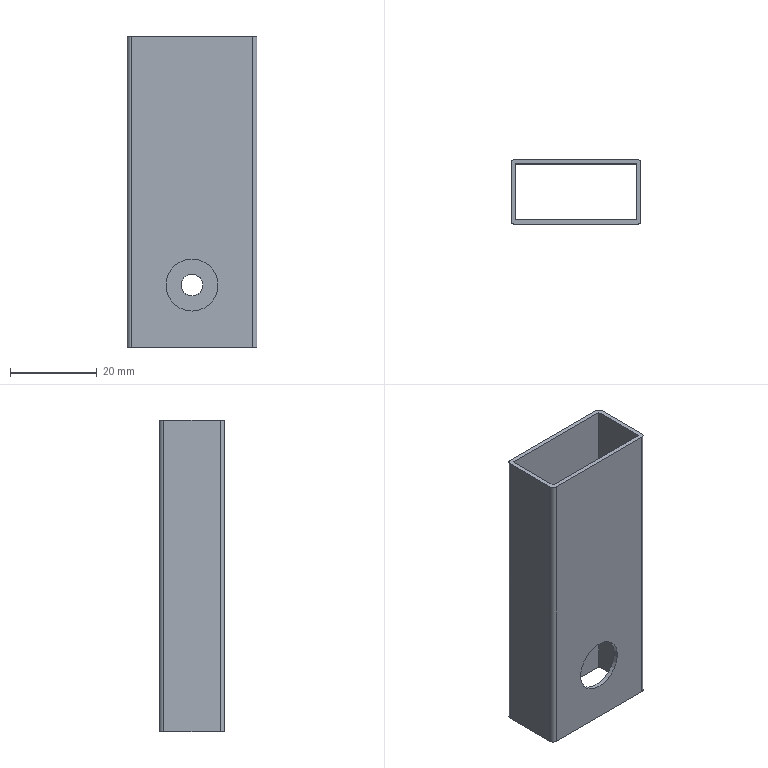Part | STEP file | Q7C1201 | 1 solid | 16 faces | box 30 x 15 x 72 mm | volume 5997 mm3 | plane 10 | cylinder 6 | commonest cylinder face diameters 2 x4 5 x1 12 x1
STEP:
#1=CARTESIAN_POINT('',(0.,0.,0.));
#2=DIRECTION('',(0.,0.,1.));
#3=DIRECTION('',(1.,0.,0.));
#4=AXIS2_PLACEMENT_3D('',#1,#2,#3);
#5=CARTESIAN_POINT('',(15.,6.5,36.));
#6=VERTEX_POINT('',#5);
#7=CARTESIAN_POINT('',(14.,7.5,36.));
#8=VERTEX_POINT('',#7);
#9=CARTESIAN_POINT('',(14.,6.5,36.));
#10=DIRECTION('',(0.,0.,1.));
#11=DIRECTION('',(-1.,0.,0.));
#12=AXIS2_PLACEMENT_3D('',#9,#10,#11);
#13=CIRCLE('',#12,1.);
#14=CARTESIAN_POINT('',(14.,6.5,36.));
#15=DIRECTION('',(0.,0.,-1.));
#16=DIRECTION('',(-1.,0.,0.));
#17=AXIS2_PLACEMENT_3D('',#14,#15,#16);
#18=PLANE('',#17);
#19=CARTESIAN_POINT('',(1.,0.));
#20=CARTESIAN_POINT('',(1.,-1.732));
#21=CARTESIAN_POINT('',(-0.5,-0.866));
#22=CARTESIAN_POINT('',(-2.,0.));
#23=CARTESIAN_POINT('',(-0.5,0.866));
#24=CARTESIAN_POINT('',(1.,1.732));
#25=CARTESIAN_POINT('',(1.,0.));
#26=(BOUNDED_CURVE()B_SPLINE_CURVE(2,(#19,#20,#21,#22,#23,#24,#25),.UNSPECIFIED.,.T.,.F.)B_SPLINE_CURVE_WITH_KNOTS((1,2,2,2,2,1),(-2.094,0.,2.094,4.189,6.283,8.378),.UNSPECIFIED.)CURVE()GEOMETRIC_REPRESENTATION_ITEM()RATIONAL_B_SPLINE_CURVE((1.,0.5,1.,0.5,1.,0.5,1.))REPRESENTATION_ITEM(''));
#27=(GEOMETRIC_REPRESENTATION_CONTEXT(2)PARAMETRIC_REPRESENTATION_CONTEXT()REPRESENTATION_CONTEXT('',''));
#28=DEFINITIONAL_REPRESENTATION('',(#26),#27);
#29=PCURVE('',#18,#28);
#30=CARTESIAN_POINT('',(14.,6.5,36.));
#31=DIRECTION('',(0.,0.,-1.));
#32=DIRECTION('',(-1.,0.,0.));
#33=AXIS2_PLACEMENT_3D('',#30,#31,#32);
#34=CYLINDRICAL_SURFACE('',#33,1.);
#35=CARTESIAN_POINT('',(6.283,0.));
#36=DIRECTION('',(-1.,0.));
#37=VECTOR('',#36,1.);
#38=LINE('',#35,#37);
#39=(GEOMETRIC_REPRESENTATION_CONTEXT(2)PARAMETRIC_REPRESENTATION_CONTEXT()REPRESENTATION_CONTEXT('',''));
#40=DEFINITIONAL_REPRESENTATION('',(#38),#39);
#41=PCURVE('',#34,#40);
#42=SURFACE_CURVE('',#13,(#29,#41),.PCURVE_S1.);
#43=EDGE_CURVE('',#6,#8,#42,.T.);
#44=ORIENTED_EDGE('',*,*,#43,.T.);
#45=CARTESIAN_POINT('',(-14.,7.5,36.));
#46=VERTEX_POINT('',#45);
#47=CARTESIAN_POINT('',(-14.,7.5,36.));
#48=DIRECTION('',(-1.,0.,0.));
#49=VECTOR('',#48,1.);
#50=LINE('',#47,#49);
#51=CARTESIAN_POINT('',(28.,1.));
#52=DIRECTION('',(1.,0.));
#53=VECTOR('',#52,1.);
#54=LINE('',#51,#53);
#55=(GEOMETRIC_REPRESENTATION_CONTEXT(2)PARAMETRIC_REPRESENTATION_CONTEXT()REPRESENTATION_CONTEXT('',''));
#56=DEFINITIONAL_REPRESENTATION('',(#54),#55);
#57=PCURVE('',#18,#56);
#58=CARTESIAN_POINT('',(-14.,7.5,36.));
#59=DIRECTION('',(0.,-1.,0.));
#60=DIRECTION('',(0.,0.,-1.));
#61=AXIS2_PLACEMENT_3D('',#58,#59,#60);
#62=PLANE('',#61);
#63=CARTESIAN_POINT('',(0.,0.));
#64=DIRECTION('',(0.,-1.));
#65=VECTOR('',#64,1.);
#66=LINE('',#63,#65);
#67=(GEOMETRIC_REPRESENTATION_CONTEXT(2)PARAMETRIC_REPRESENTATION_CONTEXT()REPRESENTATION_CONTEXT('',''));
#68=DEFINITIONAL_REPRESENTATION('',(#66),#67);
#69=PCURVE('',#62,#68);
#70=SURFACE_CURVE('',#50,(#57,#69),.PCURVE_S1.);
#71=EDGE_CURVE('',#8,#46,#70,.T.);
#72=ORIENTED_EDGE('',*,*,#71,.T.);
#73=CARTESIAN_POINT('',(-15.,6.5,36.));
#74=VERTEX_POINT('',#73);
#75=CARTESIAN_POINT('',(-14.,6.5,36.));
#76=DIRECTION('',(0.,0.,1.));
#77=DIRECTION('',(1.,0.,0.));
#78=AXIS2_PLACEMENT_3D('',#75,#76,#77);
#79=CIRCLE('',#78,1.);
#80=CARTESIAN_POINT('',(27.,0.));
#81=CARTESIAN_POINT('',(27.,1.732));
#82=CARTESIAN_POINT('',(28.5,0.866));
#83=CARTESIAN_POINT('',(30.,0.));
#84=CARTESIAN_POINT('',(28.5,-0.866));
#85=CARTESIAN_POINT('',(27.,-1.732));
#86=CARTESIAN_POINT('',(27.,0.));
#87=(BOUNDED_CURVE()B_SPLINE_CURVE(2,(#80,#81,#82,#83,#84,#85,#86),.UNSPECIFIED.,.T.,.F.)B_SPLINE_CURVE_WITH_KNOTS((1,2,2,2,2,1),(-2.094,0.,2.094,4.189,6.283,8.378),.UNSPECIFIED.)CURVE()GEOMETRIC_REPRESENTATION_ITEM()RATIONAL_B_SPLINE_CURVE((1.,0.5,1.,0.5,1.,0.5,1.))REPRESENTATION_ITEM(''));
#88=(GEOMETRIC_REPRESENTATION_CONTEXT(2)PARAMETRIC_REPRESENTATION_CONTEXT()REPRESENTATION_CONTEXT('',''));
#89=DEFINITIONAL_REPRESENTATION('',(#87),#88);
#90=PCURVE('',#18,#89);
#91=CARTESIAN_POINT('',(-14.,6.5,36.));
#92=DIRECTION('',(0.,0.,-1.));
#93=DIRECTION('',(-1.,0.,0.));
#94=AXIS2_PLACEMENT_3D('',#91,#92,#93);
#95=CYLINDRICAL_SURFACE('',#94,1.);
#96=CARTESIAN_POINT('',(3.142,0.));
#97=DIRECTION('',(-1.,0.));
#98=VECTOR('',#97,1.);
#99=LINE('',#96,#98);
#100=(GEOMETRIC_REPRESENTATION_CONTEXT(2)PARAMETRIC_REPRESENTATION_CONTEXT()REPRESENTATION_CONTEXT('',''));
#101=DEFINITIONAL_REPRESENTATION('',(#99),#100);
#102=PCURVE('',#95,#101);
#103=SURFACE_CURVE('',#79,(#90,#102),.PCURVE_S1.);
#104=EDGE_CURVE('',#46,#74,#103,.T.);
#105=ORIENTED_EDGE('',*,*,#104,.T.);
#106=CARTESIAN_POINT('',(-15.,-6.5,36.));
#107=VERTEX_POINT('',#106);
#108=CARTESIAN_POINT('',(-15.,6.5,36.));
#109=DIRECTION('',(0.,-1.,0.));
#110=VECTOR('',#109,1.);
#111=LINE('',#108,#110);
#112=CARTESIAN_POINT('',(29.,0.));
#113=DIRECTION('',(0.,-1.));
#114=VECTOR('',#113,1.);
#115=LINE('',#112,#114);
#116=(GEOMETRIC_REPRESENTATION_CONTEXT(2)PARAMETRIC_REPRESENTATION_CONTEXT()REPRESENTATION_CONTEXT('',''));
#117=DEFINITIONAL_REPRESENTATION('',(#115),#116);
#118=PCURVE('',#18,#117);
#119=CARTESIAN_POINT('',(-15.,6.5,36.));
#120=DIRECTION('',(1.,0.,0.));
#121=DIRECTION('',(0.,1.,0.));
#122=AXIS2_PLACEMENT_3D('',#119,#120,#121);
#123=PLANE('',#122);
#124=CARTESIAN_POINT('',(0.,0.));
#125=DIRECTION('',(-1.,0.));
#126=VECTOR('',#125,1.);
#127=LINE('',#124,#126);
#128=(GEOMETRIC_REPRESENTATION_CONTEXT(2)PARAMETRIC_REPRESENTATION_CONTEXT()REPRESENTATION_CONTEXT('',''));
#129=DEFINITIONAL_REPRESENTATION('',(#127),#128);
#130=PCURVE('',#123,#129);
#131=SURFACE_CURVE('',#111,(#118,#130),.PCURVE_S1.);
#132=EDGE_CURVE('',#74,#107,#131,.T.);
#133=ORIENTED_EDGE('',*,*,#132,.T.);
#134=CARTESIAN_POINT('',(-14.,-7.5,36.));
#135=VERTEX_POINT('',#134);
#136=CARTESIAN_POINT('',(-14.,-6.5,36.));
#137=DIRECTION('',(0.,0.,1.));
#138=DIRECTION('',(1.,0.,0.));
#139=AXIS2_PLACEMENT_3D('',#136,#137,#138);
#140=CIRCLE('',#139,1.);
#141=CARTESIAN_POINT('',(27.,-13.));
#142=CARTESIAN_POINT('',(27.,-11.268));
#143=CARTESIAN_POINT('',(28.5,-12.134));
#144=CARTESIAN_POINT('',(30.,-13.));
#145=CARTESIAN_POINT('',(28.5,-13.866));
#146=CARTESIAN_POINT('',(27.,-14.732));
#147=CARTESIAN_POINT('',(27.,-13.));
#148=(BOUNDED_CURVE()B_SPLINE_CURVE(2,(#141,#142,#143,#144,#145,#146,#147),.UNSPECIFIED.,.T.,.F.)B_SPLINE_CURVE_WITH_KNOTS((1,2,2,2,2,1),(-2.094,0.,2.094,4.189,6.283,8.378),.UNSPECIFIED.)CURVE()GEOMETRIC_REPRESENTATION_ITEM()RATIONAL_B_SPLINE_CURVE((1.,0.5,1.,0.5,1.,0.5,1.))REPRESENTATION_ITEM(''));
#149=(GEOMETRIC_REPRESENTATION_CONTEXT(2)PARAMETRIC_REPRESENTATION_CONTEXT()REPRESENTATION_CONTEXT('',''));
#150=DEFINITIONAL_REPRESENTATION('',(#148),#149);
#151=PCURVE('',#18,#150);
#152=CARTESIAN_POINT('',(-14.,-6.5,36.));
#153=DIRECTION('',(0.,0.,-1.));
#154=DIRECTION('',(-1.,0.,0.));
#155=AXIS2_PLACEMENT_3D('',#152,#153,#154);
#156=CYLINDRICAL_SURFACE('',#155,1.);
#157=CARTESIAN_POINT('',(9.425,0.));
#158=DIRECTION('',(-1.,0.));
#159=VECTOR('',#158,1.);
#160=LINE('',#157,#159);
#161=(GEOMETRIC_REPRESENTATION_CONTEXT(2)PARAMETRIC_REPRESENTATION_CONTEXT()REPRESENTATION_CONTEXT('',''));
#162=DEFINITIONAL_REPRESENTATION('',(#160),#161);
#163=PCURVE('',#156,#162);
#164=SURFACE_CURVE('',#140,(#151,#163),.PCURVE_S1.);
#165=EDGE_CURVE('',#107,#135,#164,.T.);
#166=ORIENTED_EDGE('',*,*,#165,.T.);
#167=CARTESIAN_POINT('',(14.,-7.5,36.));
#168=VERTEX_POINT('',#167);
#169=CARTESIAN_POINT('',(-14.,-7.5,36.));
#170=DIRECTION('',(1.,0.,0.));
#171=VECTOR('',#170,1.);
#172=LINE('',#169,#171);
#173=CARTESIAN_POINT('',(28.,-14.));
#174=DIRECTION('',(-1.,0.));
#175=VECTOR('',#174,1.);
#176=LINE('',#173,#175);
#177=(GEOMETRIC_REPRESENTATION_CONTEXT(2)PARAMETRIC_REPRESENTATION_CONTEXT()REPRESENTATION_CONTEXT('',''));
#178=DEFINITIONAL_REPRESENTATION('',(#176),#177);
#179=PCURVE('',#18,#178);
#180=CARTESIAN_POINT('',(-14.,-7.5,36.));
#181=DIRECTION('',(0.,1.,0.));
#182=DIRECTION('',(0.,0.,1.));
#183=AXIS2_PLACEMENT_3D('',#180,#181,#182);
#184=PLANE('',#183);
#185=CARTESIAN_POINT('',(0.,0.));
#186=DIRECTION('',(0.,1.));
#187=VECTOR('',#186,1.);
#188=LINE('',#185,#187);
#189=(GEOMETRIC_REPRESENTATION_CONTEXT(2)PARAMETRIC_REPRESENTATION_CONTEXT()REPRESENTATION_CONTEXT('',''));
#190=DEFINITIONAL_REPRESENTATION('',(#188),#189);
#191=PCURVE('',#184,#190);
#192=SURFACE_CURVE('',#172,(#179,#191),.PCURVE_S1.);
#193=EDGE_CURVE('',#135,#168,#192,.T.);
#194=ORIENTED_EDGE('',*,*,#193,.T.);
#195=CARTESIAN_POINT('',(15.,-6.5,36.));
#196=VERTEX_POINT('',#195);
#197=CARTESIAN_POINT('',(14.,-6.5,36.));
#198=DIRECTION('',(0.,0.,1.));
#199=DIRECTION('',(1.,0.,0.));
#200=AXIS2_PLACEMENT_3D('',#197,#198,#199);
#201=CIRCLE('',#200,1.);
#202=CARTESIAN_POINT('',(-1.,-13.));
#203=CARTESIAN_POINT('',(-1.,-11.268));
#204=CARTESIAN_POINT('',(0.5,-12.134));
#205=CARTESIAN_POINT('',(2.,-13.));
#206=CARTESIAN_POINT('',(0.5,-13.866));
#207=CARTESIAN_POINT('',(-1.,-14.732));
#208=CARTESIAN_POINT('',(-1.,-13.));
#209=(BOUNDED_CURVE()B_SPLINE_CURVE(2,(#202,#203,#204,#205,#206,#207,#208),.UNSPECIFIED.,.T.,.F.)B_SPLINE_CURVE_WITH_KNOTS((1,2,2,2,2,1),(-2.094,0.,2.094,4.189,6.283,8.378),.UNSPECIFIED.)CURVE()GEOMETRIC_REPRESENTATION_ITEM()RATIONAL_B_SPLINE_CURVE((1.,0.5,1.,0.5,1.,0.5,1.))REPRESENTATION_ITEM(''));
#210=(GEOMETRIC_REPRESENTATION_CONTEXT(2)PARAMETRIC_REPRESENTATION_CONTEXT()REPRESENTATION_CONTEXT('',''));
#211=DEFINITIONAL_REPRESENTATION('',(#209),#210);
#212=PCURVE('',#18,#211);
#213=CARTESIAN_POINT('',(14.,-6.5,36.));
#214=DIRECTION('',(0.,0.,-1.));
#215=DIRECTION('',(-1.,0.,0.));
#216=AXIS2_PLACEMENT_3D('',#213,#214,#215);
#217=CYLINDRICAL_SURFACE('',#216,1.);
#218=CARTESIAN_POINT('',(9.425,0.));
#219=DIRECTION('',(-1.,0.));
#220=VECTOR('',#219,1.);
#221=LINE('',#218,#220);
#222=(GEOMETRIC_REPRESENTATION_CONTEXT(2)PARAMETRIC_REPRESENTATION_CONTEXT()REPRESENTATION_CONTEXT('',''));
#223=DEFINITIONAL_REPRESENTATION('',(#221),#222);
#224=PCURVE('',#217,#223);
#225=SURFACE_CURVE('',#201,(#212,#224),.PCURVE_S1.);
#226=EDGE_CURVE('',#168,#196,#225,.T.);
#227=ORIENTED_EDGE('',*,*,#226,.T.);
#228=CARTESIAN_POINT('',(15.,6.5,36.));
#229=DIRECTION('',(0.,1.,0.));
#230=VECTOR('',#229,1.);
#231=LINE('',#228,#230);
#232=CARTESIAN_POINT('',(-1.,0.));
#233=DIRECTION('',(0.,1.));
#234=VECTOR('',#233,1.);
#235=LINE('',#232,#234);
#236=(GEOMETRIC_REPRESENTATION_CONTEXT(2)PARAMETRIC_REPRESENTATION_CONTEXT()REPRESENTATION_CONTEXT('',''));
#237=DEFINITIONAL_REPRESENTATION('',(#235),#236);
#238=PCURVE('',#18,#237);
#239=CARTESIAN_POINT('',(15.,6.5,36.));
#240=DIRECTION('',(-1.,0.,0.));
#241=DIRECTION('',(0.,0.,1.));
#242=AXIS2_PLACEMENT_3D('',#239,#240,#241);
#243=PLANE('',#242);
#244=CARTESIAN_POINT('',(0.,0.));
#245=DIRECTION('',(0.,1.));
#246=VECTOR('',#245,1.);
#247=LINE('',#244,#246);
#248=(GEOMETRIC_REPRESENTATION_CONTEXT(2)PARAMETRIC_REPRESENTATION_CONTEXT()REPRESENTATION_CONTEXT('',''));
#249=DEFINITIONAL_REPRESENTATION('',(#247),#248);
#250=PCURVE('',#243,#249);
#251=SURFACE_CURVE('',#231,(#238,#250),.PCURVE_S1.);
#252=EDGE_CURVE('',#196,#6,#251,.T.);
#253=ORIENTED_EDGE('',*,*,#252,.T.);
#254=EDGE_LOOP('',(#44,#72,#105,#133,#166,#194,#227,#253));
#255=FACE_BOUND('',#254,.T.);
#256=CARTESIAN_POINT('',(14.,6.5,36.));
#257=VERTEX_POINT('',#256);
#258=CARTESIAN_POINT('',(-14.,6.5,36.));
#259=VERTEX_POINT('',#258);
#260=CARTESIAN_POINT('',(-14.,6.5,36.));
#261=DIRECTION('',(-1.,0.,0.));
#262=VECTOR('',#261,1.);
#263=LINE('',#260,#262);
#264=CARTESIAN_POINT('',(28.,0.));
#265=DIRECTION('',(1.,0.));
#266=VECTOR('',#265,1.);
#267=LINE('',#264,#266);
#268=(GEOMETRIC_REPRESENTATION_CONTEXT(2)PARAMETRIC_REPRESENTATION_CONTEXT()REPRESENTATION_CONTEXT('',''));
#269=DEFINITIONAL_REPRESENTATION('',(#267),#268);
#270=PCURVE('',#18,#269);
#271=CARTESIAN_POINT('',(-14.,6.5,36.));
#272=DIRECTION('',(0.,-1.,0.));
#273=DIRECTION('',(0.,0.,-1.));
#274=AXIS2_PLACEMENT_3D('',#271,#272,#273);
#275=PLANE('',#274);
#276=CARTESIAN_POINT('',(0.,0.));
#277=DIRECTION('',(0.,-1.));
#278=VECTOR('',#277,1.);
#279=LINE('',#276,#278);
#280=(GEOMETRIC_REPRESENTATION_CONTEXT(2)PARAMETRIC_REPRESENTATION_CONTEXT()REPRESENTATION_CONTEXT('',''));
#281=DEFINITIONAL_REPRESENTATION('',(#279),#280);
#282=PCURVE('',#275,#281);
#283=SURFACE_CURVE('',#263,(#270,#282),.PCURVE_S1.);
#284=EDGE_CURVE('',#257,#259,#283,.T.);
#285=ORIENTED_EDGE('',*,*,#284,.F.);
#286=CARTESIAN_POINT('',(14.,-6.5,36.));
#287=VERTEX_POINT('',#286);
#288=CARTESIAN_POINT('',(14.,6.5,36.));
#289=DIRECTION('',(0.,1.,0.));
#290=VECTOR('',#289,1.);
#291=LINE('',#288,#290);
#292=CARTESIAN_POINT('',(0.,0.));
#293=DIRECTION('',(0.,1.));
#294=VECTOR('',#293,1.);
#295=LINE('',#292,#294);
#296=(GEOMETRIC_REPRESENTATION_CONTEXT(2)PARAMETRIC_REPRESENTATION_CONTEXT()REPRESENTATION_CONTEXT('',''));
#297=DEFINITIONAL_REPRESENTATION('',(#295),#296);
#298=PCURVE('',#18,#297);
#299=CARTESIAN_POINT('',(14.,6.5,36.));
#300=DIRECTION('',(-1.,0.,0.));
#301=DIRECTION('',(0.,-1.,0.));
#302=AXIS2_PLACEMENT_3D('',#299,#300,#301);
#303=PLANE('',#302);
#304=CARTESIAN_POINT('',(0.,0.));
#305=DIRECTION('',(-1.,0.));
#306=VECTOR('',#305,1.);
#307=LINE('',#304,#306);
#308=(GEOMETRIC_REPRESENTATION_CONTEXT(2)PARAMETRIC_REPRESENTATION_CONTEXT()REPRESENTATION_CONTEXT('',''));
#309=DEFINITIONAL_REPRESENTATION('',(#307),#308);
#310=PCURVE('',#303,#309);
#311=SURFACE_CURVE('',#291,(#298,#310),.PCURVE_S1.);
#312=EDGE_CURVE('',#287,#257,#311,.T.);
#313=ORIENTED_EDGE('',*,*,#312,.F.);
#314=CARTESIAN_POINT('',(-14.,-6.5,36.));
#315=VERTEX_POINT('',#314);
#316=CARTESIAN_POINT('',(-14.,-6.5,36.));
#317=DIRECTION('',(1.,0.,0.));
#318=VECTOR('',#317,1.);
#319=LINE('',#316,#318);
#320=CARTESIAN_POINT('',(28.,-13.));
#321=DIRECTION('',(-1.,0.));
#322=VECTOR('',#321,1.);
#323=LINE('',#320,#322);
#324=(GEOMETRIC_REPRESENTATION_CONTEXT(2)PARAMETRIC_REPRESENTATION_CONTEXT()REPRESENTATION_CONTEXT('',''));
#325=DEFINITIONAL_REPRESENTATION('',(#323),#324);
#326=PCURVE('',#18,#325);
#327=CARTESIAN_POINT('',(-14.,-6.5,36.));
#328=DIRECTION('',(0.,1.,0.));
#329=DIRECTION('',(0.,0.,1.));
#330=AXIS2_PLACEMENT_3D('',#327,#328,#329);
#331=PLANE('',#330);
#332=CARTESIAN_POINT('',(0.,0.));
#333=DIRECTION('',(0.,1.));
#334=VECTOR('',#333,1.);
#335=LINE('',#332,#334);
#336=(GEOMETRIC_REPRESENTATION_CONTEXT(2)PARAMETRIC_REPRESENTATION_CONTEXT()REPRESENTATION_CONTEXT('',''));
#337=DEFINITIONAL_REPRESENTATION('',(#335),#336);
#338=PCURVE('',#331,#337);
#339=SURFACE_CURVE('',#319,(#326,#338),.PCURVE_S1.);
#340=EDGE_CURVE('',#315,#287,#339,.T.);
#341=ORIENTED_EDGE('',*,*,#340,.F.);
#342=CARTESIAN_POINT('',(-14.,6.5,36.));
#343=DIRECTION('',(0.,-1.,0.));
#344=VECTOR('',#343,1.);
#345=LINE('',#342,#344);
#346=CARTESIAN_POINT('',(28.,0.));
#347=DIRECTION('',(0.,-1.));
#348=VECTOR('',#347,1.);
#349=LINE('',#346,#348);
#350=(GEOMETRIC_REPRESENTATION_CONTEXT(2)PARAMETRIC_REPRESENTATION_CONTEXT()REPRESENTATION_CONTEXT('',''));
#351=DEFINITIONAL_REPRESENTATION('',(#349),#350);
#352=PCURVE('',#18,#351);
#353=CARTESIAN_POINT('',(-14.,6.5,36.));
#354=DIRECTION('',(1.,0.,0.));
#355=DIRECTION('',(0.,1.,0.));
#356=AXIS2_PLACEMENT_3D('',#353,#354,#355);
#357=PLANE('',#356);
#358=CARTESIAN_POINT('',(0.,0.));
#359=DIRECTION('',(-1.,0.));
#360=VECTOR('',#359,1.);
#361=LINE('',#358,#360);
#362=(GEOMETRIC_REPRESENTATION_CONTEXT(2)PARAMETRIC_REPRESENTATION_CONTEXT()REPRESENTATION_CONTEXT('',''));
#363=DEFINITIONAL_REPRESENTATION('',(#361),#362);
#364=PCURVE('',#357,#363);
#365=SURFACE_CURVE('',#345,(#352,#364),.PCURVE_S1.);
#366=EDGE_CURVE('',#259,#315,#365,.T.);
#367=ORIENTED_EDGE('',*,*,#366,.F.);
#368=EDGE_LOOP('',(#285,#313,#341,#367));
#369=FACE_BOUND('',#368,.T.);
#370=ADVANCED_FACE('',(#255,#369),#18,.F.);
#371=CARTESIAN_POINT('',(15.,6.5,-36.));
#372=VERTEX_POINT('',#371);
#373=CARTESIAN_POINT('',(14.,7.5,-36.));
#374=VERTEX_POINT('',#373);
#375=CARTESIAN_POINT('',(14.,6.5,-36.));
#376=DIRECTION('',(0.,0.,1.));
#377=DIRECTION('',(-1.,0.,0.));
#378=AXIS2_PLACEMENT_3D('',#375,#376,#377);
#379=CIRCLE('',#378,1.);
#380=CARTESIAN_POINT('',(14.,6.5,-36.));
#381=DIRECTION('',(0.,0.,-1.));
#382=DIRECTION('',(-1.,0.,0.));
#383=AXIS2_PLACEMENT_3D('',#380,#381,#382);
#384=PLANE('',#383);
#385=CARTESIAN_POINT('',(1.,0.));
#386=CARTESIAN_POINT('',(1.,-1.732));
#387=CARTESIAN_POINT('',(-0.5,-0.866));
#388=CARTESIAN_POINT('',(-2.,0.));
#389=CARTESIAN_POINT('',(-0.5,0.866));
#390=CARTESIAN_POINT('',(1.,1.732));
#391=CARTESIAN_POINT('',(1.,0.));
#392=(BOUNDED_CURVE()B_SPLINE_CURVE(2,(#385,#386,#387,#388,#389,#390,#391),.UNSPECIFIED.,.T.,.F.)B_SPLINE_CURVE_WITH_KNOTS((1,2,2,2,2,1),(-2.094,0.,2.094,4.189,6.283,8.378),.UNSPECIFIED.)CURVE()GEOMETRIC_REPRESENTATION_ITEM()RATIONAL_B_SPLINE_CURVE((1.,0.5,1.,0.5,1.,0.5,1.))REPRESENTATION_ITEM(''));
#393=(GEOMETRIC_REPRESENTATION_CONTEXT(2)PARAMETRIC_REPRESENTATION_CONTEXT()REPRESENTATION_CONTEXT('',''));
#394=DEFINITIONAL_REPRESENTATION('',(#392),#393);
#395=PCURVE('',#384,#394);
#396=CARTESIAN_POINT('',(6.283,72.));
#397=DIRECTION('',(-1.,0.));
#398=VECTOR('',#397,1.);
#399=LINE('',#396,#398);
#400=(GEOMETRIC_REPRESENTATION_CONTEXT(2)PARAMETRIC_REPRESENTATION_CONTEXT()REPRESENTATION_CONTEXT('',''));
#401=DEFINITIONAL_REPRESENTATION('',(#399),#400);
#402=PCURVE('',#34,#401);
#403=SURFACE_CURVE('',#379,(#395,#402),.PCURVE_S1.);
#404=EDGE_CURVE('',#372,#374,#403,.T.);
#405=ORIENTED_EDGE('',*,*,#404,.F.);
#406=CARTESIAN_POINT('',(15.,-6.5,-36.));
#407=VERTEX_POINT('',#406);
#408=CARTESIAN_POINT('',(15.,6.5,-36.));
#409=DIRECTION('',(0.,1.,0.));
#410=VECTOR('',#409,1.);
#411=LINE('',#408,#410);
#412=CARTESIAN_POINT('',(-1.,0.));
#413=DIRECTION('',(0.,1.));
#414=VECTOR('',#413,1.);
#415=LINE('',#412,#414);
#416=(GEOMETRIC_REPRESENTATION_CONTEXT(2)PARAMETRIC_REPRESENTATION_CONTEXT()REPRESENTATION_CONTEXT('',''));
#417=DEFINITIONAL_REPRESENTATION('',(#415),#416);
#418=PCURVE('',#384,#417);
#419=CARTESIAN_POINT('',(-72.,0.));
#420=DIRECTION('',(0.,1.));
#421=VECTOR('',#420,1.);
#422=LINE('',#419,#421);
#423=(GEOMETRIC_REPRESENTATION_CONTEXT(2)PARAMETRIC_REPRESENTATION_CONTEXT()REPRESENTATION_CONTEXT('',''));
#424=DEFINITIONAL_REPRESENTATION('',(#422),#423);
#425=PCURVE('',#243,#424);
#426=SURFACE_CURVE('',#411,(#418,#425),.PCURVE_S1.);
#427=EDGE_CURVE('',#407,#372,#426,.T.);
#428=ORIENTED_EDGE('',*,*,#427,.F.);
#429=CARTESIAN_POINT('',(14.,-7.5,-36.));
#430=VERTEX_POINT('',#429);
#431=CARTESIAN_POINT('',(14.,-6.5,-36.));
#432=DIRECTION('',(0.,0.,1.));
#433=DIRECTION('',(1.,0.,0.));
#434=AXIS2_PLACEMENT_3D('',#431,#432,#433);
#435=CIRCLE('',#434,1.);
#436=CARTESIAN_POINT('',(-1.,-13.));
#437=CARTESIAN_POINT('',(-1.,-11.268));
#438=CARTESIAN_POINT('',(0.5,-12.134));
#439=CARTESIAN_POINT('',(2.,-13.));
#440=CARTESIAN_POINT('',(0.5,-13.866));
#441=CARTESIAN_POINT('',(-1.,-14.732));
#442=CARTESIAN_POINT('',(-1.,-13.));
#443=(BOUNDED_CURVE()B_SPLINE_CURVE(2,(#436,#437,#438,#439,#440,#441,#442),.UNSPECIFIED.,.T.,.F.)B_SPLINE_CURVE_WITH_KNOTS((1,2,2,2,2,1),(-2.094,0.,2.094,4.189,6.283,8.378),.UNSPECIFIED.)CURVE()GEOMETRIC_REPRESENTATION_ITEM()RATIONAL_B_SPLINE_CURVE((1.,0.5,1.,0.5,1.,0.5,1.))REPRESENTATION_ITEM(''));
#444=(GEOMETRIC_REPRESENTATION_CONTEXT(2)PARAMETRIC_REPRESENTATION_CONTEXT()REPRESENTATION_CONTEXT('',''));
#445=DEFINITIONAL_REPRESENTATION('',(#443),#444);
#446=PCURVE('',#384,#445);
#447=CARTESIAN_POINT('',(9.425,72.));
#448=DIRECTION('',(-1.,0.));
#449=VECTOR('',#448,1.);
#450=LINE('',#447,#449);
#451=(GEOMETRIC_REPRESENTATION_CONTEXT(2)PARAMETRIC_REPRESENTATION_CONTEXT()REPRESENTATION_CONTEXT('',''));
#452=DEFINITIONAL_REPRESENTATION('',(#450),#451);
#453=PCURVE('',#217,#452);
#454=SURFACE_CURVE('',#435,(#446,#453),.PCURVE_S1.);
#455=EDGE_CURVE('',#430,#407,#454,.T.);
#456=ORIENTED_EDGE('',*,*,#455,.F.);
#457=CARTESIAN_POINT('',(-14.,-7.5,-36.));
#458=VERTEX_POINT('',#457);
#459=CARTESIAN_POINT('',(-14.,-7.5,-36.));
#460=DIRECTION('',(1.,0.,0.));
#461=VECTOR('',#460,1.);
#462=LINE('',#459,#461);
#463=CARTESIAN_POINT('',(28.,-14.));
#464=DIRECTION('',(-1.,0.));
#465=VECTOR('',#464,1.);
#466=LINE('',#463,#465);
#467=(GEOMETRIC_REPRESENTATION_CONTEXT(2)PARAMETRIC_REPRESENTATION_CONTEXT()REPRESENTATION_CONTEXT('',''));
#468=DEFINITIONAL_REPRESENTATION('',(#466),#467);
#469=PCURVE('',#384,#468);
#470=CARTESIAN_POINT('',(-72.,0.));
#471=DIRECTION('',(0.,1.));
#472=VECTOR('',#471,1.);
#473=LINE('',#470,#472);
#474=(GEOMETRIC_REPRESENTATION_CONTEXT(2)PARAMETRIC_REPRESENTATION_CONTEXT()REPRESENTATION_CONTEXT('',''));
#475=DEFINITIONAL_REPRESENTATION('',(#473),#474);
#476=PCURVE('',#184,#475);
#477=SURFACE_CURVE('',#462,(#469,#476),.PCURVE_S1.);
#478=EDGE_CURVE('',#458,#430,#477,.T.);
#479=ORIENTED_EDGE('',*,*,#478,.F.);
#480=CARTESIAN_POINT('',(-15.,-6.5,-36.));
#481=VERTEX_POINT('',#480);
#482=CARTESIAN_POINT('',(-14.,-6.5,-36.));
#483=DIRECTION('',(0.,0.,1.));
#484=DIRECTION('',(1.,0.,0.));
#485=AXIS2_PLACEMENT_3D('',#482,#483,#484);
#486=CIRCLE('',#485,1.);
#487=CARTESIAN_POINT('',(27.,-13.));
#488=CARTESIAN_POINT('',(27.,-11.268));
#489=CARTESIAN_POINT('',(28.5,-12.134));
#490=CARTESIAN_POINT('',(30.,-13.));
#491=CARTESIAN_POINT('',(28.5,-13.866));
#492=CARTESIAN_POINT('',(27.,-14.732));
#493=CARTESIAN_POINT('',(27.,-13.));
#494=(BOUNDED_CURVE()B_SPLINE_CURVE(2,(#487,#488,#489,#490,#491,#492,#493),.UNSPECIFIED.,.T.,.F.)B_SPLINE_CURVE_WITH_KNOTS((1,2,2,2,2,1),(-2.094,0.,2.094,4.189,6.283,8.378),.UNSPECIFIED.)CURVE()GEOMETRIC_REPRESENTATION_ITEM()RATIONAL_B_SPLINE_CURVE((1.,0.5,1.,0.5,1.,0.5,1.))REPRESENTATION_ITEM(''));
#495=(GEOMETRIC_REPRESENTATION_CONTEXT(2)PARAMETRIC_REPRESENTATION_CONTEXT()REPRESENTATION_CONTEXT('',''));
#496=DEFINITIONAL_REPRESENTATION('',(#494),#495);
#497=PCURVE('',#384,#496);
#498=CARTESIAN_POINT('',(9.425,72.));
#499=DIRECTION('',(-1.,0.));
#500=VECTOR('',#499,1.);
#501=LINE('',#498,#500);
#502=(GEOMETRIC_REPRESENTATION_CONTEXT(2)PARAMETRIC_REPRESENTATION_CONTEXT()REPRESENTATION_CONTEXT('',''));
#503=DEFINITIONAL_REPRESENTATION('',(#501),#502);
#504=PCURVE('',#156,#503);
#505=SURFACE_CURVE('',#486,(#497,#504),.PCURVE_S1.);
#506=EDGE_CURVE('',#481,#458,#505,.T.);
#507=ORIENTED_EDGE('',*,*,#506,.F.);
#508=CARTESIAN_POINT('',(-15.,6.5,-36.));
#509=VERTEX_POINT('',#508);
#510=CARTESIAN_POINT('',(-15.,6.5,-36.));
#511=DIRECTION('',(0.,-1.,0.));
#512=VECTOR('',#511,1.);
#513=LINE('',#510,#512);
#514=CARTESIAN_POINT('',(29.,0.));
#515=DIRECTION('',(0.,-1.));
#516=VECTOR('',#515,1.);
#517=LINE('',#514,#516);
#518=(GEOMETRIC_REPRESENTATION_CONTEXT(2)PARAMETRIC_REPRESENTATION_CONTEXT()REPRESENTATION_CONTEXT('',''));
#519=DEFINITIONAL_REPRESENTATION('',(#517),#518);
#520=PCURVE('',#384,#519);
#521=CARTESIAN_POINT('',(0.,-72.));
#522=DIRECTION('',(-1.,0.));
#523=VECTOR('',#522,1.);
#524=LINE('',#521,#523);
#525=(GEOMETRIC_REPRESENTATION_CONTEXT(2)PARAMETRIC_REPRESENTATION_CONTEXT()REPRESENTATION_CONTEXT('',''));
#526=DEFINITIONAL_REPRESENTATION('',(#524),#525);
#527=PCURVE('',#123,#526);
#528=SURFACE_CURVE('',#513,(#520,#527),.PCURVE_S1.);
#529=EDGE_CURVE('',#509,#481,#528,.T.);
#530=ORIENTED_EDGE('',*,*,#529,.F.);
#531=CARTESIAN_POINT('',(-14.,7.5,-36.));
#532=VERTEX_POINT('',#531);
#533=CARTESIAN_POINT('',(-14.,6.5,-36.));
#534=DIRECTION('',(0.,0.,1.));
#535=DIRECTION('',(1.,0.,0.));
#536=AXIS2_PLACEMENT_3D('',#533,#534,#535);
#537=CIRCLE('',#536,1.);
#538=CARTESIAN_POINT('',(27.,0.));
#539=CARTESIAN_POINT('',(27.,1.732));
#540=CARTESIAN_POINT('',(28.5,0.866));
#541=CARTESIAN_POINT('',(30.,0.));
#542=CARTESIAN_POINT('',(28.5,-0.866));
#543=CARTESIAN_POINT('',(27.,-1.732));
#544=CARTESIAN_POINT('',(27.,0.));
#545=(BOUNDED_CURVE()B_SPLINE_CURVE(2,(#538,#539,#540,#541,#542,#543,#544),.UNSPECIFIED.,.T.,.F.)B_SPLINE_CURVE_WITH_KNOTS((1,2,2,2,2,1),(-2.094,0.,2.094,4.189,6.283,8.378),.UNSPECIFIED.)CURVE()GEOMETRIC_REPRESENTATION_ITEM()RATIONAL_B_SPLINE_CURVE((1.,0.5,1.,0.5,1.,0.5,1.))REPRESENTATION_ITEM(''));
#546=(GEOMETRIC_REPRESENTATION_CONTEXT(2)PARAMETRIC_REPRESENTATION_CONTEXT()REPRESENTATION_CONTEXT('',''));
#547=DEFINITIONAL_REPRESENTATION('',(#545),#546);
#548=PCURVE('',#384,#547);
#549=CARTESIAN_POINT('',(3.142,72.));
#550=DIRECTION('',(-1.,0.));
#551=VECTOR('',#550,1.);
#552=LINE('',#549,#551);
#553=(GEOMETRIC_REPRESENTATION_CONTEXT(2)PARAMETRIC_REPRESENTATION_CONTEXT()REPRESENTATION_CONTEXT('',''));
#554=DEFINITIONAL_REPRESENTATION('',(#552),#553);
#555=PCURVE('',#95,#554);
#556=SURFACE_CURVE('',#537,(#548,#555),.PCURVE_S1.);
#557=EDGE_CURVE('',#532,#509,#556,.T.);
#558=ORIENTED_EDGE('',*,*,#557,.F.);
#559=CARTESIAN_POINT('',(-14.,7.5,-36.));
#560=DIRECTION('',(-1.,0.,0.));
#561=VECTOR('',#560,1.);
#562=LINE('',#559,#561);
#563=CARTESIAN_POINT('',(28.,1.));
#564=DIRECTION('',(1.,0.));
#565=VECTOR('',#564,1.);
#566=LINE('',#563,#565);
#567=(GEOMETRIC_REPRESENTATION_CONTEXT(2)PARAMETRIC_REPRESENTATION_CONTEXT()REPRESENTATION_CONTEXT('',''));
#568=DEFINITIONAL_REPRESENTATION('',(#566),#567);
#569=PCURVE('',#384,#568);
#570=CARTESIAN_POINT('',(72.,0.));
#571=DIRECTION('',(0.,-1.));
#572=VECTOR('',#571,1.);
#573=LINE('',#570,#572);
#574=(GEOMETRIC_REPRESENTATION_CONTEXT(2)PARAMETRIC_REPRESENTATION_CONTEXT()REPRESENTATION_CONTEXT('',''));
#575=DEFINITIONAL_REPRESENTATION('',(#573),#574);
#576=PCURVE('',#62,#575);
#577=SURFACE_CURVE('',#562,(#569,#576),.PCURVE_S1.);
#578=EDGE_CURVE('',#374,#532,#577,.T.);
#579=ORIENTED_EDGE('',*,*,#578,.F.);
#580=EDGE_LOOP('',(#405,#428,#456,#479,#507,#530,#558,#579));
#581=FACE_BOUND('',#580,.T.);
#582=CARTESIAN_POINT('',(14.,-6.5,-36.));
#583=VERTEX_POINT('',#582);
#584=CARTESIAN_POINT('',(14.,6.5,-36.));
#585=VERTEX_POINT('',#584);
#586=CARTESIAN_POINT('',(14.,6.5,-36.));
#587=DIRECTION('',(0.,1.,0.));
#588=VECTOR('',#587,1.);
#589=LINE('',#586,#588);
#590=CARTESIAN_POINT('',(0.,0.));
#591=DIRECTION('',(0.,1.));
#592=VECTOR('',#591,1.);
#593=LINE('',#590,#592);
#594=(GEOMETRIC_REPRESENTATION_CONTEXT(2)PARAMETRIC_REPRESENTATION_CONTEXT()REPRESENTATION_CONTEXT('',''));
#595=DEFINITIONAL_REPRESENTATION('',(#593),#594);
#596=PCURVE('',#384,#595);
#597=CARTESIAN_POINT('',(0.,-72.));
#598=DIRECTION('',(-1.,0.));
#599=VECTOR('',#598,1.);
#600=LINE('',#597,#599);
#601=(GEOMETRIC_REPRESENTATION_CONTEXT(2)PARAMETRIC_REPRESENTATION_CONTEXT()REPRESENTATION_CONTEXT('',''));
#602=DEFINITIONAL_REPRESENTATION('',(#600),#601);
#603=PCURVE('',#303,#602);
#604=SURFACE_CURVE('',#589,(#596,#603),.PCURVE_S1.);
#605=EDGE_CURVE('',#583,#585,#604,.T.);
#606=ORIENTED_EDGE('',*,*,#605,.T.);
#607=CARTESIAN_POINT('',(-14.,6.5,-36.));
#608=VERTEX_POINT('',#607);
#609=CARTESIAN_POINT('',(-14.,6.5,-36.));
#610=DIRECTION('',(-1.,0.,0.));
#611=VECTOR('',#610,1.);
#612=LINE('',#609,#611);
#613=CARTESIAN_POINT('',(28.,0.));
#614=DIRECTION('',(1.,0.));
#615=VECTOR('',#614,1.);
#616=LINE('',#613,#615);
#617=(GEOMETRIC_REPRESENTATION_CONTEXT(2)PARAMETRIC_REPRESENTATION_CONTEXT()REPRESENTATION_CONTEXT('',''));
#618=DEFINITIONAL_REPRESENTATION('',(#616),#617);
#619=PCURVE('',#384,#618);
#620=CARTESIAN_POINT('',(72.,0.));
#621=DIRECTION('',(0.,-1.));
#622=VECTOR('',#621,1.);
#623=LINE('',#620,#622);
#624=(GEOMETRIC_REPRESENTATION_CONTEXT(2)PARAMETRIC_REPRESENTATION_CONTEXT()REPRESENTATION_CONTEXT('',''));
#625=DEFINITIONAL_REPRESENTATION('',(#623),#624);
#626=PCURVE('',#275,#625);
#627=SURFACE_CURVE('',#612,(#619,#626),.PCURVE_S1.);
#628=EDGE_CURVE('',#585,#608,#627,.T.);
#629=ORIENTED_EDGE('',*,*,#628,.T.);
#630=CARTESIAN_POINT('',(-14.,-6.5,-36.));
#631=VERTEX_POINT('',#630);
#632=CARTESIAN_POINT('',(-14.,6.5,-36.));
#633=DIRECTION('',(0.,-1.,0.));
#634=VECTOR('',#633,1.);
#635=LINE('',#632,#634);
#636=CARTESIAN_POINT('',(28.,0.));
#637=DIRECTION('',(0.,-1.));
#638=VECTOR('',#637,1.);
#639=LINE('',#636,#638);
#640=(GEOMETRIC_REPRESENTATION_CONTEXT(2)PARAMETRIC_REPRESENTATION_CONTEXT()REPRESENTATION_CONTEXT('',''));
#641=DEFINITIONAL_REPRESENTATION('',(#639),#640);
#642=PCURVE('',#384,#641);
#643=CARTESIAN_POINT('',(0.,-72.));
#644=DIRECTION('',(-1.,0.));
#645=VECTOR('',#644,1.);
#646=LINE('',#643,#645);
#647=(GEOMETRIC_REPRESENTATION_CONTEXT(2)PARAMETRIC_REPRESENTATION_CONTEXT()REPRESENTATION_CONTEXT('',''));
#648=DEFINITIONAL_REPRESENTATION('',(#646),#647);
#649=PCURVE('',#357,#648);
#650=SURFACE_CURVE('',#635,(#642,#649),.PCURVE_S1.);
#651=EDGE_CURVE('',#608,#631,#650,.T.);
#652=ORIENTED_EDGE('',*,*,#651,.T.);
#653=CARTESIAN_POINT('',(-14.,-6.5,-36.));
#654=DIRECTION('',(1.,0.,0.));
#655=VECTOR('',#654,1.);
#656=LINE('',#653,#655);
#657=CARTESIAN_POINT('',(28.,-13.));
#658=DIRECTION('',(-1.,0.));
#659=VECTOR('',#658,1.);
#660=LINE('',#657,#659);
#661=(GEOMETRIC_REPRESENTATION_CONTEXT(2)PARAMETRIC_REPRESENTATION_CONTEXT()REPRESENTATION_CONTEXT('',''));
#662=DEFINITIONAL_REPRESENTATION('',(#660),#661);
#663=PCURVE('',#384,#662);
#664=CARTESIAN_POINT('',(-72.,0.));
#665=DIRECTION('',(0.,1.));
#666=VECTOR('',#665,1.);
#667=LINE('',#664,#666);
#668=(GEOMETRIC_REPRESENTATION_CONTEXT(2)PARAMETRIC_REPRESENTATION_CONTEXT()REPRESENTATION_CONTEXT('',''));
#669=DEFINITIONAL_REPRESENTATION('',(#667),#668);
#670=PCURVE('',#331,#669);
#671=SURFACE_CURVE('',#656,(#663,#670),.PCURVE_S1.);
#672=EDGE_CURVE('',#631,#583,#671,.T.);
#673=ORIENTED_EDGE('',*,*,#672,.T.);
#674=EDGE_LOOP('',(#606,#629,#652,#673));
#675=FACE_BOUND('',#674,.T.);
#676=ADVANCED_FACE('',(#581,#675),#384,.T.);
#677=ORIENTED_EDGE('',*,*,#404,.T.);
#678=CARTESIAN_POINT('',(14.,7.5,36.));
#679=DIRECTION('',(0.,0.,-1.));
#680=VECTOR('',#679,1.);
#681=LINE('',#678,#680);
#682=CARTESIAN_POINT('',(1.571,0.));
#683=DIRECTION('',(0.,1.));
#684=VECTOR('',#683,1.);
#685=LINE('',#682,#684);
#686=(GEOMETRIC_REPRESENTATION_CONTEXT(2)PARAMETRIC_REPRESENTATION_CONTEXT()REPRESENTATION_CONTEXT('',''));
#687=DEFINITIONAL_REPRESENTATION('',(#685),#686);
#688=PCURVE('',#34,#687);
#689=CARTESIAN_POINT('',(0.,28.));
#690=DIRECTION('',(1.,0.));
#691=VECTOR('',#690,1.);
#692=LINE('',#689,#691);
#693=(GEOMETRIC_REPRESENTATION_CONTEXT(2)PARAMETRIC_REPRESENTATION_CONTEXT()REPRESENTATION_CONTEXT('',''));
#694=DEFINITIONAL_REPRESENTATION('',(#692),#693);
#695=PCURVE('',#62,#694);
#696=SURFACE_CURVE('',#681,(#688,#695),.PCURVE_S1.);
#697=EDGE_CURVE('',#8,#374,#696,.T.);
#698=ORIENTED_EDGE('',*,*,#697,.F.);
#699=ORIENTED_EDGE('',*,*,#43,.F.);
#700=CARTESIAN_POINT('',(15.,6.5,36.));
#701=DIRECTION('',(0.,0.,-1.));
#702=VECTOR('',#701,1.);
#703=LINE('',#700,#702);
#704=CARTESIAN_POINT('',(3.142,0.));
#705=DIRECTION('',(0.,1.));
#706=VECTOR('',#705,1.);
#707=LINE('',#704,#706);
#708=(GEOMETRIC_REPRESENTATION_CONTEXT(2)PARAMETRIC_REPRESENTATION_CONTEXT()REPRESENTATION_CONTEXT('',''));
#709=DEFINITIONAL_REPRESENTATION('',(#707),#708);
#710=PCURVE('',#34,#709);
#711=CARTESIAN_POINT('',(0.,0.));
#712=DIRECTION('',(-1.,0.));
#713=VECTOR('',#712,1.);
#714=LINE('',#711,#713);
#715=(GEOMETRIC_REPRESENTATION_CONTEXT(2)PARAMETRIC_REPRESENTATION_CONTEXT()REPRESENTATION_CONTEXT('',''));
#716=DEFINITIONAL_REPRESENTATION('',(#714),#715);
#717=PCURVE('',#243,#716);
#718=SURFACE_CURVE('',#703,(#710,#717),.PCURVE_S1.);
#719=EDGE_CURVE('',#6,#372,#718,.T.);
#720=ORIENTED_EDGE('',*,*,#719,.T.);
#721=EDGE_LOOP('',(#677,#698,#699,#720));
#722=FACE_BOUND('',#721,.T.);
#723=ADVANCED_FACE('',(#722),#34,.T.);
#724=CARTESIAN_POINT('',(0.,7.5,-24.));
#725=VERTEX_POINT('',#724);
#726=CARTESIAN_POINT('',(2.5,7.5,-21.5));
#727=VERTEX_POINT('',#726);
#728=CARTESIAN_POINT('',(0.,7.5,-21.5));
#729=DIRECTION('',(0.,-1.,0.));
#730=DIRECTION('',(0.,0.,-1.));
#731=AXIS2_PLACEMENT_3D('',#728,#729,#730);
#732=CIRCLE('',#731,2.5);
#733=CARTESIAN_POINT('',(57.5,14.));
#734=DIRECTION('',(1.,0.));
#735=AXIS2_PLACEMENT_2D('',#733,#734);
#736=CIRCLE('',#735,2.5);
#737=(GEOMETRIC_REPRESENTATION_CONTEXT(2)PARAMETRIC_REPRESENTATION_CONTEXT()REPRESENTATION_CONTEXT('',''));
#738=DEFINITIONAL_REPRESENTATION('',(#736),#737);
#739=PCURVE('',#62,#738);
#740=CARTESIAN_POINT('',(0.,9.5,-21.5));
#741=DIRECTION('',(0.,-1.,0.));
#742=DIRECTION('',(1.,0.,0.));
#743=AXIS2_PLACEMENT_3D('',#740,#741,#742);
#744=CYLINDRICAL_SURFACE('',#743,2.5);
#745=CARTESIAN_POINT('',(4.712,2.));
#746=DIRECTION('',(1.,0.));
#747=VECTOR('',#746,1.);
#748=LINE('',#745,#747);
#749=(GEOMETRIC_REPRESENTATION_CONTEXT(2)PARAMETRIC_REPRESENTATION_CONTEXT()REPRESENTATION_CONTEXT('',''));
#750=DEFINITIONAL_REPRESENTATION('',(#748),#749);
#751=PCURVE('',#744,#750);
#752=SURFACE_CURVE('',#732,(#739,#751),.PCURVE_S1.);
#753=EDGE_CURVE('',#725,#727,#752,.T.);
#754=ORIENTED_EDGE('',*,*,#753,.T.);
#755=CARTESIAN_POINT('',(0.,7.5,-21.5));
#756=DIRECTION('',(0.,-1.,0.));
#757=DIRECTION('',(0.,0.,-1.));
#758=AXIS2_PLACEMENT_3D('',#755,#756,#757);
#759=CIRCLE('',#758,2.5);
#760=CARTESIAN_POINT('',(57.5,14.));
#761=DIRECTION('',(1.,0.));
#762=AXIS2_PLACEMENT_2D('',#760,#761);
#763=CIRCLE('',#762,2.5);
#764=(GEOMETRIC_REPRESENTATION_CONTEXT(2)PARAMETRIC_REPRESENTATION_CONTEXT()REPRESENTATION_CONTEXT('',''));
#765=DEFINITIONAL_REPRESENTATION('',(#763),#764);
#766=PCURVE('',#62,#765);
#767=CARTESIAN_POINT('',(-1.571,2.));
#768=DIRECTION('',(1.,0.));
#769=VECTOR('',#768,1.);
#770=LINE('',#767,#769);
#771=(GEOMETRIC_REPRESENTATION_CONTEXT(2)PARAMETRIC_REPRESENTATION_CONTEXT()REPRESENTATION_CONTEXT('',''));
#772=DEFINITIONAL_REPRESENTATION('',(#770),#771);
#773=PCURVE('',#744,#772);
#774=SURFACE_CURVE('',#759,(#766,#773),.PCURVE_S1.);
#775=EDGE_CURVE('',#727,#725,#774,.T.);
#776=ORIENTED_EDGE('',*,*,#775,.T.);
#777=EDGE_LOOP('',(#754,#776));
#778=FACE_BOUND('',#777,.T.);
#779=ORIENTED_EDGE('',*,*,#578,.T.);
#780=CARTESIAN_POINT('',(-14.,7.5,36.));
#781=DIRECTION('',(0.,0.,-1.));
#782=VECTOR('',#781,1.);
#783=LINE('',#780,#782);
#784=CARTESIAN_POINT('',(0.,0.));
#785=DIRECTION('',(1.,0.));
#786=VECTOR('',#785,1.);
#787=LINE('',#784,#786);
#788=(GEOMETRIC_REPRESENTATION_CONTEXT(2)PARAMETRIC_REPRESENTATION_CONTEXT()REPRESENTATION_CONTEXT('',''));
#789=DEFINITIONAL_REPRESENTATION('',(#787),#788);
#790=PCURVE('',#62,#789);
#791=CARTESIAN_POINT('',(1.571,0.));
#792=DIRECTION('',(0.,1.));
#793=VECTOR('',#792,1.);
#794=LINE('',#791,#793);
#795=(GEOMETRIC_REPRESENTATION_CONTEXT(2)PARAMETRIC_REPRESENTATION_CONTEXT()REPRESENTATION_CONTEXT('',''));
#796=DEFINITIONAL_REPRESENTATION('',(#794),#795);
#797=PCURVE('',#95,#796);
#798=SURFACE_CURVE('',#783,(#790,#797),.PCURVE_S1.);
#799=EDGE_CURVE('',#46,#532,#798,.T.);
#800=ORIENTED_EDGE('',*,*,#799,.F.);
#801=ORIENTED_EDGE('',*,*,#71,.F.);
#802=ORIENTED_EDGE('',*,*,#697,.T.);
#803=EDGE_LOOP('',(#779,#800,#801,#802));
#804=FACE_BOUND('',#803,.T.);
#805=ADVANCED_FACE('',(#778,#804),#62,.F.);
#806=ORIENTED_EDGE('',*,*,#557,.T.);
#807=CARTESIAN_POINT('',(-15.,6.5,36.));
#808=DIRECTION('',(0.,0.,-1.));
#809=VECTOR('',#808,1.);
#810=LINE('',#807,#809);
#811=CARTESIAN_POINT('',(0.,0.));
#812=DIRECTION('',(0.,1.));
#813=VECTOR('',#812,1.);
#814=LINE('',#811,#813);
#815=(GEOMETRIC_REPRESENTATION_CONTEXT(2)PARAMETRIC_REPRESENTATION_CONTEXT()REPRESENTATION_CONTEXT('',''));
#816=DEFINITIONAL_REPRESENTATION('',(#814),#815);
#817=PCURVE('',#95,#816);
#818=CARTESIAN_POINT('',(0.,0.));
#819=DIRECTION('',(0.,-1.));
#820=VECTOR('',#819,1.);
#821=LINE('',#818,#820);
#822=(GEOMETRIC_REPRESENTATION_CONTEXT(2)PARAMETRIC_REPRESENTATION_CONTEXT()REPRESENTATION_CONTEXT('',''));
#823=DEFINITIONAL_REPRESENTATION('',(#821),#822);
#824=PCURVE('',#123,#823);
#825=SURFACE_CURVE('',#810,(#817,#824),.PCURVE_S1.);
#826=EDGE_CURVE('',#74,#509,#825,.T.);
#827=ORIENTED_EDGE('',*,*,#826,.F.);
#828=ORIENTED_EDGE('',*,*,#104,.F.);
#829=ORIENTED_EDGE('',*,*,#799,.T.);
#830=EDGE_LOOP('',(#806,#827,#828,#829));
#831=FACE_BOUND('',#830,.T.);
#832=ADVANCED_FACE('',(#831),#95,.T.);
#833=ORIENTED_EDGE('',*,*,#529,.T.);
#834=CARTESIAN_POINT('',(-15.,-6.5,36.));
#835=DIRECTION('',(0.,0.,-1.));
#836=VECTOR('',#835,1.);
#837=LINE('',#834,#836);
#838=CARTESIAN_POINT('',(-13.,0.));
#839=DIRECTION('',(0.,-1.));
#840=VECTOR('',#839,1.);
#841=LINE('',#838,#840);
#842=(GEOMETRIC_REPRESENTATION_CONTEXT(2)PARAMETRIC_REPRESENTATION_CONTEXT()REPRESENTATION_CONTEXT('',''));
#843=DEFINITIONAL_REPRESENTATION('',(#841),#842);
#844=PCURVE('',#123,#843);
#845=CARTESIAN_POINT('',(6.283,0.));
#846=DIRECTION('',(0.,1.));
#847=VECTOR('',#846,1.);
#848=LINE('',#845,#847);
#849=(GEOMETRIC_REPRESENTATION_CONTEXT(2)PARAMETRIC_REPRESENTATION_CONTEXT()REPRESENTATION_CONTEXT('',''));
#850=DEFINITIONAL_REPRESENTATION('',(#848),#849);
#851=PCURVE('',#156,#850);
#852=SURFACE_CURVE('',#837,(#844,#851),.PCURVE_S1.);
#853=EDGE_CURVE('',#107,#481,#852,.T.);
#854=ORIENTED_EDGE('',*,*,#853,.F.);
#855=ORIENTED_EDGE('',*,*,#132,.F.);
#856=ORIENTED_EDGE('',*,*,#826,.T.);
#857=EDGE_LOOP('',(#833,#854,#855,#856));
#858=FACE_BOUND('',#857,.T.);
#859=ADVANCED_FACE('',(#858),#123,.F.);
#860=ORIENTED_EDGE('',*,*,#506,.T.);
#861=CARTESIAN_POINT('',(-14.,-7.5,36.));
#862=DIRECTION('',(0.,0.,-1.));
#863=VECTOR('',#862,1.);
#864=LINE('',#861,#863);
#865=CARTESIAN_POINT('',(4.712,0.));
#866=DIRECTION('',(0.,1.));
#867=VECTOR('',#866,1.);
#868=LINE('',#865,#867);
#869=(GEOMETRIC_REPRESENTATION_CONTEXT(2)PARAMETRIC_REPRESENTATION_CONTEXT()REPRESENTATION_CONTEXT('',''));
#870=DEFINITIONAL_REPRESENTATION('',(#868),#869);
#871=PCURVE('',#156,#870);
#872=CARTESIAN_POINT('',(0.,0.));
#873=DIRECTION('',(-1.,0.));
#874=VECTOR('',#873,1.);
#875=LINE('',#872,#874);
#876=(GEOMETRIC_REPRESENTATION_CONTEXT(2)PARAMETRIC_REPRESENTATION_CONTEXT()REPRESENTATION_CONTEXT('',''));
#877=DEFINITIONAL_REPRESENTATION('',(#875),#876);
#878=PCURVE('',#184,#877);
#879=SURFACE_CURVE('',#864,(#871,#878),.PCURVE_S1.);
#880=EDGE_CURVE('',#135,#458,#879,.T.);
#881=ORIENTED_EDGE('',*,*,#880,.F.);
#882=ORIENTED_EDGE('',*,*,#165,.F.);
#883=ORIENTED_EDGE('',*,*,#853,.T.);
#884=EDGE_LOOP('',(#860,#881,#882,#883));
#885=FACE_BOUND('',#884,.T.);
#886=ADVANCED_FACE('',(#885),#156,.T.);
#887=CARTESIAN_POINT('',(0.,-7.5,-27.5));
#888=VERTEX_POINT('',#887);
#889=CARTESIAN_POINT('',(0.,-7.5,-21.5));
#890=DIRECTION('',(0.,-1.,0.));
#891=DIRECTION('',(0.,0.,-1.));
#892=AXIS2_PLACEMENT_3D('',#889,#890,#891);
#893=CIRCLE('',#892,6.);
#894=CARTESIAN_POINT('',(-63.5,14.));
#895=CARTESIAN_POINT('',(-63.5,24.392));
#896=CARTESIAN_POINT('',(-54.5,19.196));
#897=CARTESIAN_POINT('',(-45.5,14.));
#898=CARTESIAN_POINT('',(-54.5,8.804));
#899=CARTESIAN_POINT('',(-63.5,3.608));
#900=CARTESIAN_POINT('',(-63.5,14.));
#901=(BOUNDED_CURVE()B_SPLINE_CURVE(2,(#894,#895,#896,#897,#898,#899,#900),.UNSPECIFIED.,.T.,.F.)B_SPLINE_CURVE_WITH_KNOTS((1,2,2,2,2,1),(-2.094,0.,2.094,4.189,6.283,8.378),.UNSPECIFIED.)CURVE()GEOMETRIC_REPRESENTATION_ITEM()RATIONAL_B_SPLINE_CURVE((1.,0.5,1.,0.5,1.,0.5,1.))REPRESENTATION_ITEM(''));
#902=(GEOMETRIC_REPRESENTATION_CONTEXT(2)PARAMETRIC_REPRESENTATION_CONTEXT()REPRESENTATION_CONTEXT('',''));
#903=DEFINITIONAL_REPRESENTATION('',(#901),#902);
#904=PCURVE('',#184,#903);
#905=CARTESIAN_POINT('',(0.,-4.5,-21.5));
#906=DIRECTION('',(0.,-1.,0.));
#907=DIRECTION('',(0.,0.,-1.));
#908=AXIS2_PLACEMENT_3D('',#905,#906,#907);
#909=CYLINDRICAL_SURFACE('',#908,6.);
#910=CARTESIAN_POINT('',(0.,3.));
#911=DIRECTION('',(1.,0.));
#912=VECTOR('',#911,1.);
#913=LINE('',#910,#912);
#914=(GEOMETRIC_REPRESENTATION_CONTEXT(2)PARAMETRIC_REPRESENTATION_CONTEXT()REPRESENTATION_CONTEXT('',''));
#915=DEFINITIONAL_REPRESENTATION('',(#913),#914);
#916=PCURVE('',#909,#915);
#917=SURFACE_CURVE('',#893,(#904,#916),.PCURVE_S1.);
#918=EDGE_CURVE('',#888,#888,#917,.T.);
#919=ORIENTED_EDGE('',*,*,#918,.F.);
#920=EDGE_LOOP('',(#919));
#921=FACE_BOUND('',#920,.T.);
#922=ORIENTED_EDGE('',*,*,#478,.T.);
#923=CARTESIAN_POINT('',(14.,-7.5,36.));
#924=DIRECTION('',(0.,0.,-1.));
#925=VECTOR('',#924,1.);
#926=LINE('',#923,#925);
#927=CARTESIAN_POINT('',(0.,28.));
#928=DIRECTION('',(-1.,0.));
#929=VECTOR('',#928,1.);
#930=LINE('',#927,#929);
#931=(GEOMETRIC_REPRESENTATION_CONTEXT(2)PARAMETRIC_REPRESENTATION_CONTEXT()REPRESENTATION_CONTEXT('',''));
#932=DEFINITIONAL_REPRESENTATION('',(#930),#931);
#933=PCURVE('',#184,#932);
#934=CARTESIAN_POINT('',(4.712,0.));
#935=DIRECTION('',(0.,1.));
#936=VECTOR('',#935,1.);
#937=LINE('',#934,#936);
#938=(GEOMETRIC_REPRESENTATION_CONTEXT(2)PARAMETRIC_REPRESENTATION_CONTEXT()REPRESENTATION_CONTEXT('',''));
#939=DEFINITIONAL_REPRESENTATION('',(#937),#938);
#940=PCURVE('',#217,#939);
#941=SURFACE_CURVE('',#926,(#933,#940),.PCURVE_S1.);
#942=EDGE_CURVE('',#168,#430,#941,.T.);
#943=ORIENTED_EDGE('',*,*,#942,.F.);
#944=ORIENTED_EDGE('',*,*,#193,.F.);
#945=ORIENTED_EDGE('',*,*,#880,.T.);
#946=EDGE_LOOP('',(#922,#943,#944,#945));
#947=FACE_BOUND('',#946,.T.);
#948=ADVANCED_FACE('',(#921,#947),#184,.F.);
#949=ORIENTED_EDGE('',*,*,#455,.T.);
#950=CARTESIAN_POINT('',(15.,-6.5,36.));
#951=DIRECTION('',(0.,0.,-1.));
#952=VECTOR('',#951,1.);
#953=LINE('',#950,#952);
#954=CARTESIAN_POINT('',(3.142,0.));
#955=DIRECTION('',(0.,1.));
#956=VECTOR('',#955,1.);
#957=LINE('',#954,#956);
#958=(GEOMETRIC_REPRESENTATION_CONTEXT(2)PARAMETRIC_REPRESENTATION_CONTEXT()REPRESENTATION_CONTEXT('',''));
#959=DEFINITIONAL_REPRESENTATION('',(#957),#958);
#960=PCURVE('',#217,#959);
#961=CARTESIAN_POINT('',(0.,-13.));
#962=DIRECTION('',(-1.,0.));
#963=VECTOR('',#962,1.);
#964=LINE('',#961,#963);
#965=(GEOMETRIC_REPRESENTATION_CONTEXT(2)PARAMETRIC_REPRESENTATION_CONTEXT()REPRESENTATION_CONTEXT('',''));
#966=DEFINITIONAL_REPRESENTATION('',(#964),#965);
#967=PCURVE('',#243,#966);
#968=SURFACE_CURVE('',#953,(#960,#967),.PCURVE_S1.);
#969=EDGE_CURVE('',#196,#407,#968,.T.);
#970=ORIENTED_EDGE('',*,*,#969,.F.);
#971=ORIENTED_EDGE('',*,*,#226,.F.);
#972=ORIENTED_EDGE('',*,*,#942,.T.);
#973=EDGE_LOOP('',(#949,#970,#971,#972));
#974=FACE_BOUND('',#973,.T.);
#975=ADVANCED_FACE('',(#974),#217,.T.);
#976=ORIENTED_EDGE('',*,*,#427,.T.);
#977=ORIENTED_EDGE('',*,*,#719,.F.);
#978=ORIENTED_EDGE('',*,*,#252,.F.);
#979=ORIENTED_EDGE('',*,*,#969,.T.);
#980=EDGE_LOOP('',(#976,#977,#978,#979));
#981=FACE_BOUND('',#980,.T.);
#982=ADVANCED_FACE('',(#981),#243,.F.);
#983=CARTESIAN_POINT('',(2.5,6.5,-21.5));
#984=VERTEX_POINT('',#983);
#985=CARTESIAN_POINT('',(0.,6.5,-21.5));
#986=DIRECTION('',(0.,-1.,0.));
#987=DIRECTION('',(1.,0.,0.));
#988=AXIS2_PLACEMENT_3D('',#985,#986,#987);
#989=CIRCLE('',#988,2.5);
#990=CARTESIAN_POINT('',(57.5,14.));
#991=DIRECTION('',(0.,1.));
#992=AXIS2_PLACEMENT_2D('',#990,#991);
#993=CIRCLE('',#992,2.5);
#994=(GEOMETRIC_REPRESENTATION_CONTEXT(2)PARAMETRIC_REPRESENTATION_CONTEXT()REPRESENTATION_CONTEXT('',''));
#995=DEFINITIONAL_REPRESENTATION('',(#993),#994);
#996=PCURVE('',#275,#995);
#997=CARTESIAN_POINT('',(0.,3.));
#998=DIRECTION('',(1.,0.));
#999=VECTOR('',#998,1.);
#1000=LINE('',#997,#999);
#1001=(GEOMETRIC_REPRESENTATION_CONTEXT(2)PARAMETRIC_REPRESENTATION_CONTEXT()REPRESENTATION_CONTEXT('',''));
#1002=DEFINITIONAL_REPRESENTATION('',(#1000),#1001);
#1003=PCURVE('',#744,#1002);
#1004=SURFACE_CURVE('',#989,(#996,#1003),.PCURVE_S1.);
#1005=EDGE_CURVE('',#984,#984,#1004,.T.);
#1006=ORIENTED_EDGE('',*,*,#1005,.F.);
#1007=EDGE_LOOP('',(#1006));
#1008=FACE_BOUND('',#1007,.T.);
#1009=ORIENTED_EDGE('',*,*,#628,.F.);
#1010=CARTESIAN_POINT('',(14.,6.5,36.));
#1011=DIRECTION('',(0.,0.,-1.));
#1012=VECTOR('',#1011,1.);
#1013=LINE('',#1010,#1012);
#1014=CARTESIAN_POINT('',(0.,28.));
#1015=DIRECTION('',(1.,0.));
#1016=VECTOR('',#1015,1.);
#1017=LINE('',#1014,#1016);
#1018=(GEOMETRIC_REPRESENTATION_CONTEXT(2)PARAMETRIC_REPRESENTATION_CONTEXT()REPRESENTATION_CONTEXT('',''));
#1019=DEFINITIONAL_REPRESENTATION('',(#1017),#1018);
#1020=PCURVE('',#275,#1019);
#1021=CARTESIAN_POINT('',(0.,0.));
#1022=DIRECTION('',(0.,-1.));
#1023=VECTOR('',#1022,1.);
#1024=LINE('',#1021,#1023);
#1025=(GEOMETRIC_REPRESENTATION_CONTEXT(2)PARAMETRIC_REPRESENTATION_CONTEXT()REPRESENTATION_CONTEXT('',''));
#1026=DEFINITIONAL_REPRESENTATION('',(#1024),#1025);
#1027=PCURVE('',#303,#1026);
#1028=SURFACE_CURVE('',#1013,(#1020,#1027),.PCURVE_S1.);
#1029=EDGE_CURVE('',#257,#585,#1028,.T.);
#1030=ORIENTED_EDGE('',*,*,#1029,.F.);
#1031=ORIENTED_EDGE('',*,*,#284,.T.);
#1032=CARTESIAN_POINT('',(-14.,6.5,36.));
#1033=DIRECTION('',(0.,0.,-1.));
#1034=VECTOR('',#1033,1.);
#1035=LINE('',#1032,#1034);
#1036=CARTESIAN_POINT('',(0.,0.));
#1037=DIRECTION('',(1.,0.));
#1038=VECTOR('',#1037,1.);
#1039=LINE('',#1036,#1038);
#1040=(GEOMETRIC_REPRESENTATION_CONTEXT(2)PARAMETRIC_REPRESENTATION_CONTEXT()REPRESENTATION_CONTEXT('',''));
#1041=DEFINITIONAL_REPRESENTATION('',(#1039),#1040);
#1042=PCURVE('',#275,#1041);
#1043=CARTESIAN_POINT('',(0.,0.));
#1044=DIRECTION('',(0.,-1.));
#1045=VECTOR('',#1044,1.);
#1046=LINE('',#1043,#1045);
#1047=(GEOMETRIC_REPRESENTATION_CONTEXT(2)PARAMETRIC_REPRESENTATION_CONTEXT()REPRESENTATION_CONTEXT('',''));
#1048=DEFINITIONAL_REPRESENTATION('',(#1046),#1047);
#1049=PCURVE('',#357,#1048);
#1050=SURFACE_CURVE('',#1035,(#1042,#1049),.PCURVE_S1.);
#1051=EDGE_CURVE('',#259,#608,#1050,.T.);
#1052=ORIENTED_EDGE('',*,*,#1051,.T.);
#1053=EDGE_LOOP('',(#1009,#1030,#1031,#1052));
#1054=FACE_BOUND('',#1053,.T.);
#1055=ADVANCED_FACE('',(#1008,#1054),#275,.T.);
#1056=ORIENTED_EDGE('',*,*,#651,.F.);
#1057=ORIENTED_EDGE('',*,*,#1051,.F.);
#1058=ORIENTED_EDGE('',*,*,#366,.T.);
#1059=CARTESIAN_POINT('',(-14.,-6.5,36.));
#1060=DIRECTION('',(0.,0.,-1.));
#1061=VECTOR('',#1060,1.);
#1062=LINE('',#1059,#1061);
#1063=CARTESIAN_POINT('',(-13.,0.));
#1064=DIRECTION('',(0.,-1.));
#1065=VECTOR('',#1064,1.);
#1066=LINE('',#1063,#1065);
#1067=(GEOMETRIC_REPRESENTATION_CONTEXT(2)PARAMETRIC_REPRESENTATION_CONTEXT()REPRESENTATION_CONTEXT('',''));
#1068=DEFINITIONAL_REPRESENTATION('',(#1066),#1067);
#1069=PCURVE('',#357,#1068);
#1070=CARTESIAN_POINT('',(0.,0.));
#1071=DIRECTION('',(-1.,0.));
#1072=VECTOR('',#1071,1.);
#1073=LINE('',#1070,#1072);
#1074=(GEOMETRIC_REPRESENTATION_CONTEXT(2)PARAMETRIC_REPRESENTATION_CONTEXT()REPRESENTATION_CONTEXT('',''));
#1075=DEFINITIONAL_REPRESENTATION('',(#1073),#1074);
#1076=PCURVE('',#331,#1075);
#1077=SURFACE_CURVE('',#1062,(#1069,#1076),.PCURVE_S1.);
#1078=EDGE_CURVE('',#315,#631,#1077,.T.);
#1079=ORIENTED_EDGE('',*,*,#1078,.T.);
#1080=EDGE_LOOP('',(#1056,#1057,#1058,#1079));
#1081=FACE_BOUND('',#1080,.T.);
#1082=ADVANCED_FACE('',(#1081),#357,.T.);
#1083=CARTESIAN_POINT('',(0.,-6.5,-15.5));
#1084=VERTEX_POINT('',#1083);
#1085=CARTESIAN_POINT('',(0.,-6.5,-27.5));
#1086=VERTEX_POINT('',#1085);
#1087=CARTESIAN_POINT('',(0.,-6.5,-21.5));
#1088=DIRECTION('',(0.,1.,0.));
#1089=DIRECTION('',(0.,0.,1.));
#1090=AXIS2_PLACEMENT_3D('',#1087,#1088,#1089);
#1091=CIRCLE('',#1090,6.);
#1092=CARTESIAN_POINT('',(-57.5,14.));
#1093=DIRECTION('',(1.,0.));
#1094=AXIS2_PLACEMENT_2D('',#1092,#1093);
#1095=CIRCLE('',#1094,6.);
#1096=(GEOMETRIC_REPRESENTATION_CONTEXT(2)PARAMETRIC_REPRESENTATION_CONTEXT()REPRESENTATION_CONTEXT('',''));
#1097=DEFINITIONAL_REPRESENTATION('',(#1095),#1096);
#1098=PCURVE('',#331,#1097);
#1099=CARTESIAN_POINT('',(3.142,2.));
#1100=DIRECTION('',(-1.,0.));
#1101=VECTOR('',#1100,1.);
#1102=LINE('',#1099,#1101);
#1103=(GEOMETRIC_REPRESENTATION_CONTEXT(2)PARAMETRIC_REPRESENTATION_CONTEXT()REPRESENTATION_CONTEXT('',''));
#1104=DEFINITIONAL_REPRESENTATION('',(#1102),#1103);
#1105=PCURVE('',#909,#1104);
#1106=SURFACE_CURVE('',#1091,(#1098,#1105),.PCURVE_S1.);
#1107=EDGE_CURVE('',#1084,#1086,#1106,.T.);
#1108=ORIENTED_EDGE('',*,*,#1107,.F.);
#1109=CARTESIAN_POINT('',(0.,-6.5,-21.5));
#1110=DIRECTION('',(0.,1.,0.));
#1111=DIRECTION('',(0.,0.,1.));
#1112=AXIS2_PLACEMENT_3D('',#1109,#1110,#1111);
#1113=CIRCLE('',#1112,6.);
#1114=CARTESIAN_POINT('',(-57.5,14.));
#1115=DIRECTION('',(1.,0.));
#1116=AXIS2_PLACEMENT_2D('',#1114,#1115);
#1117=CIRCLE('',#1116,6.);
#1118=(GEOMETRIC_REPRESENTATION_CONTEXT(2)PARAMETRIC_REPRESENTATION_CONTEXT()REPRESENTATION_CONTEXT('',''));
#1119=DEFINITIONAL_REPRESENTATION('',(#1117),#1118);
#1120=PCURVE('',#331,#1119);
#1121=CARTESIAN_POINT('',(9.425,2.));
#1122=DIRECTION('',(-1.,0.));
#1123=VECTOR('',#1122,1.);
#1124=LINE('',#1121,#1123);
#1125=(GEOMETRIC_REPRESENTATION_CONTEXT(2)PARAMETRIC_REPRESENTATION_CONTEXT()REPRESENTATION_CONTEXT('',''));
#1126=DEFINITIONAL_REPRESENTATION('',(#1124),#1125);
#1127=PCURVE('',#909,#1126);
#1128=SURFACE_CURVE('',#1113,(#1120,#1127),.PCURVE_S1.);
#1129=EDGE_CURVE('',#1086,#1084,#1128,.T.);
#1130=ORIENTED_EDGE('',*,*,#1129,.F.);
#1131=EDGE_LOOP('',(#1108,#1130));
#1132=FACE_BOUND('',#1131,.T.);
#1133=ORIENTED_EDGE('',*,*,#672,.F.);
#1134=ORIENTED_EDGE('',*,*,#1078,.F.);
#1135=ORIENTED_EDGE('',*,*,#340,.T.);
#1136=CARTESIAN_POINT('',(14.,-6.5,36.));
#1137=DIRECTION('',(0.,0.,-1.));
#1138=VECTOR('',#1137,1.);
#1139=LINE('',#1136,#1138);
#1140=CARTESIAN_POINT('',(0.,28.));
#1141=DIRECTION('',(-1.,0.));
#1142=VECTOR('',#1141,1.);
#1143=LINE('',#1140,#1142);
#1144=(GEOMETRIC_REPRESENTATION_CONTEXT(2)PARAMETRIC_REPRESENTATION_CONTEXT()REPRESENTATION_CONTEXT('',''));
#1145=DEFINITIONAL_REPRESENTATION('',(#1143),#1144);
#1146=PCURVE('',#331,#1145);
#1147=CARTESIAN_POINT('',(13.,0.));
#1148=DIRECTION('',(0.,-1.));
#1149=VECTOR('',#1148,1.);
#1150=LINE('',#1147,#1149);
#1151=(GEOMETRIC_REPRESENTATION_CONTEXT(2)PARAMETRIC_REPRESENTATION_CONTEXT()REPRESENTATION_CONTEXT('',''));
#1152=DEFINITIONAL_REPRESENTATION('',(#1150),#1151);
#1153=PCURVE('',#303,#1152);
#1154=SURFACE_CURVE('',#1139,(#1146,#1153),.PCURVE_S1.);
#1155=EDGE_CURVE('',#287,#583,#1154,.T.);
#1156=ORIENTED_EDGE('',*,*,#1155,.T.);
#1157=EDGE_LOOP('',(#1133,#1134,#1135,#1156));
#1158=FACE_BOUND('',#1157,.T.);
#1159=ADVANCED_FACE('',(#1132,#1158),#331,.T.);
#1160=ORIENTED_EDGE('',*,*,#605,.F.);
#1161=ORIENTED_EDGE('',*,*,#1155,.F.);
#1162=ORIENTED_EDGE('',*,*,#312,.T.);
#1163=ORIENTED_EDGE('',*,*,#1029,.T.);
#1164=EDGE_LOOP('',(#1160,#1161,#1162,#1163));
#1165=FACE_BOUND('',#1164,.T.);
#1166=ADVANCED_FACE('',(#1165),#303,.T.);
#1167=ORIENTED_EDGE('',*,*,#1129,.F.);
#1168=CARTESIAN_POINT('',(0.,-6.5,-27.5));
#1169=CARTESIAN_POINT('',(0.,-7.5,-27.5));
#1170=B_SPLINE_CURVE_WITH_KNOTS('',1,(#1168,#1169),.UNSPECIFIED.,.F.,.F.,(2,2),(2.,3.),.PIECEWISE_BEZIER_KNOTS.);
#1171=CARTESIAN_POINT('',(6.283,0.));
#1172=DIRECTION('',(0.,1.));
#1173=VECTOR('',#1172,1.);
#1174=LINE('',#1171,#1173);
#1175=(GEOMETRIC_REPRESENTATION_CONTEXT(2)PARAMETRIC_REPRESENTATION_CONTEXT()REPRESENTATION_CONTEXT('',''));
#1176=DEFINITIONAL_REPRESENTATION('',(#1174),#1175);
#1177=PCURVE('',#909,#1176);
#1178=CARTESIAN_POINT('',(0.,0.));
#1179=DIRECTION('',(0.,1.));
#1180=VECTOR('',#1179,1.);
#1181=LINE('',#1178,#1180);
#1182=(GEOMETRIC_REPRESENTATION_CONTEXT(2)PARAMETRIC_REPRESENTATION_CONTEXT()REPRESENTATION_CONTEXT('',''));
#1183=DEFINITIONAL_REPRESENTATION('',(#1181),#1182);
#1184=PCURVE('',#909,#1183);
#1185=SEAM_CURVE('',#1170,(#1177,#1184),.PCURVE_S1.);
#1186=EDGE_CURVE('',#1086,#888,#1185,.T.);
#1187=ORIENTED_EDGE('',*,*,#1186,.T.);
#1188=ORIENTED_EDGE('',*,*,#918,.F.);
#1189=ORIENTED_EDGE('',*,*,#1186,.F.);
#1190=ORIENTED_EDGE('',*,*,#1107,.F.);
#1191=EDGE_LOOP('',(#1167,#1187,#1188,#1189,#1190));
#1192=FACE_BOUND('',#1191,.F.);
#1193=ADVANCED_FACE('',(#1192),#909,.F.);
#1194=ORIENTED_EDGE('',*,*,#1005,.F.);
#1195=CARTESIAN_POINT('',(2.5,7.5,-21.5));
#1196=CARTESIAN_POINT('',(2.5,6.5,-21.5));
#1197=B_SPLINE_CURVE_WITH_KNOTS('',1,(#1195,#1196),.UNSPECIFIED.,.F.,.F.,(2,2),(2.,3.),.PIECEWISE_BEZIER_KNOTS.);
#1198=CARTESIAN_POINT('',(0.,0.));
#1199=DIRECTION('',(0.,1.));
#1200=VECTOR('',#1199,1.);
#1201=LINE('',#1198,#1200);
#1202=(GEOMETRIC_REPRESENTATION_CONTEXT(2)PARAMETRIC_REPRESENTATION_CONTEXT()REPRESENTATION_CONTEXT('',''));
#1203=DEFINITIONAL_REPRESENTATION('',(#1201),#1202);
#1204=PCURVE('',#744,#1203);
#1205=CARTESIAN_POINT('',(6.283,0.));
#1206=DIRECTION('',(0.,1.));
#1207=VECTOR('',#1206,1.);
#1208=LINE('',#1205,#1207);
#1209=(GEOMETRIC_REPRESENTATION_CONTEXT(2)PARAMETRIC_REPRESENTATION_CONTEXT()REPRESENTATION_CONTEXT('',''));
#1210=DEFINITIONAL_REPRESENTATION('',(#1208),#1209);
#1211=PCURVE('',#744,#1210);
#1212=SEAM_CURVE('',#1197,(#1204,#1211),.PCURVE_S1.);
#1213=EDGE_CURVE('',#727,#984,#1212,.T.);
#1214=ORIENTED_EDGE('',*,*,#1213,.F.);
#1215=ORIENTED_EDGE('',*,*,#775,.T.);
#1216=ORIENTED_EDGE('',*,*,#753,.T.);
#1217=ORIENTED_EDGE('',*,*,#1213,.T.);
#1218=EDGE_LOOP('',(#1194,#1214,#1215,#1216,#1217));
#1219=FACE_BOUND('',#1218,.F.);
#1220=ADVANCED_FACE('',(#1219),#744,.F.);
#1221=CLOSED_SHELL('',(#370,#676,#723,#805,#832,#859,#886,#948,#975,#982,#1055,#1082,#1159,#1166,#1193,#1220));
#1222=MANIFOLD_SOLID_BREP('',#1221);
#1223=(LENGTH_UNIT()NAMED_UNIT(*)SI_UNIT(.MILLI.,.METRE.));
#1224=UNCERTAINTY_MEASURE_WITH_UNIT(LENGTH_MEASURE(0.000001),#1223,'','');
#1225=(NAMED_UNIT(*)PLANE_ANGLE_UNIT()SI_UNIT($,.RADIAN.));
#1226=(NAMED_UNIT(*)SI_UNIT($,.STERADIAN.)SOLID_ANGLE_UNIT());
#1227=(GEOMETRIC_REPRESENTATION_CONTEXT(3)GLOBAL_UNCERTAINTY_ASSIGNED_CONTEXT((#1224))GLOBAL_UNIT_ASSIGNED_CONTEXT((#1223,#1225,#1226))REPRESENTATION_CONTEXT('',''));
#1228=ADVANCED_BREP_SHAPE_REPRESENTATION('',(#4,#1222),#1227);